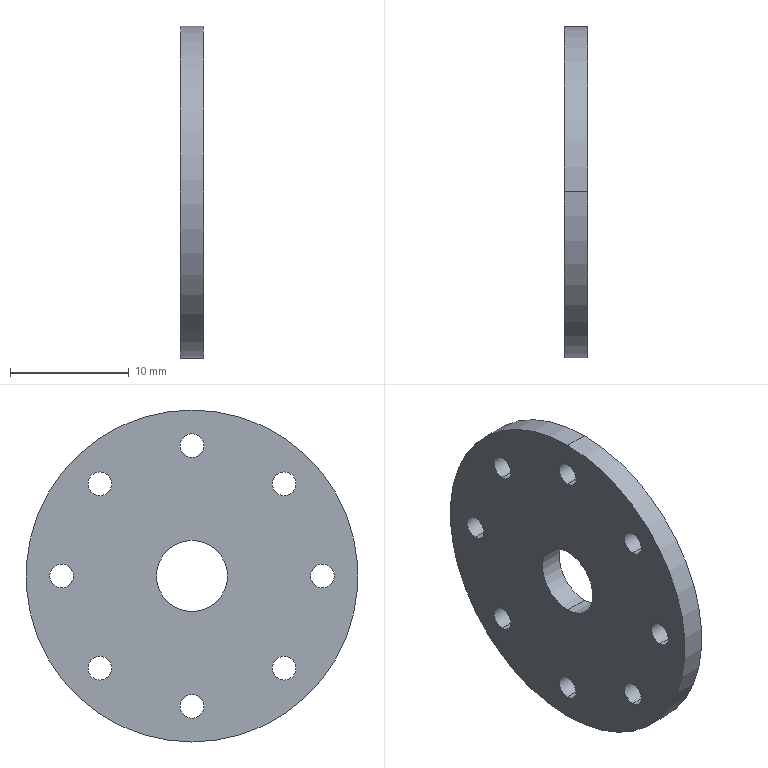Part | SolidWorks | features BaseBody 1 | 1 solid | 22 faces | box 2 x 28 x 28 mm | volume 1125 mm3 | cylinder 20 | plane 2 | commonest cylinder face diameters 2 x16 6 x2 28 x2
STEP:
#1=CARTESIAN_POINT('',(-2.,7.778,8.778));
#2=VERTEX_POINT('',#1);
#3=CARTESIAN_POINT('',(-2.,7.778,6.778));
#4=VERTEX_POINT('',#3);
#5=CARTESIAN_POINT('',(-2.,7.778,7.778));
#6=DIRECTION('',(1.,0.,0.));
#7=DIRECTION('',(0.,0.7071,-0.7071));
#8=AXIS2_PLACEMENT_3D('',#5,#6,#7);
#9=CIRCLE('',#8,1.);
#10=EDGE_CURVE('',#2,#4,#9,.T.);
#11=ORIENTED_EDGE('',*,*,#10,.F.);
#12=CARTESIAN_POINT('',(0.,7.778,8.778));
#13=VERTEX_POINT('',#12);
#14=CARTESIAN_POINT('',(-2.,7.778,8.778));
#15=DIRECTION('',(1.,0.,0.));
#16=VECTOR('',#15,1000.);
#17=LINE('',#14,#16);
#18=EDGE_CURVE('',#2,#13,#17,.T.);
#19=ORIENTED_EDGE('',*,*,#18,.T.);
#20=CARTESIAN_POINT('',(0.,7.778,6.778));
#21=VERTEX_POINT('',#20);
#22=CARTESIAN_POINT('',(0.,7.778,7.778));
#23=DIRECTION('',(1.,0.,0.));
#24=DIRECTION('',(0.,0.7071,-0.7071));
#25=AXIS2_PLACEMENT_3D('',#22,#23,#24);
#26=CIRCLE('',#25,1.);
#27=EDGE_CURVE('',#13,#21,#26,.T.);
#28=ORIENTED_EDGE('',*,*,#27,.T.);
#29=CARTESIAN_POINT('',(-2.,7.778,6.778));
#30=DIRECTION('',(1.,0.,0.));
#31=VECTOR('',#30,1000.);
#32=LINE('',#29,#31);
#33=EDGE_CURVE('',#4,#21,#32,.T.);
#34=ORIENTED_EDGE('',*,*,#33,.F.);
#35=EDGE_LOOP('',(#11,#19,#28,#34));
#36=FACE_OUTER_BOUND('',#35,.T.);
#37=CARTESIAN_POINT('',(-2.,7.778,7.778));
#38=DIRECTION('',(1.,0.,0.));
#39=DIRECTION('',(0.,0.,-1.));
#40=AXIS2_PLACEMENT_3D('',#37,#38,#39);
#41=CYLINDRICAL_SURFACE('',#40,1.);
#42=ADVANCED_FACE('',(#36),#41,.F.);
#43=CARTESIAN_POINT('',(-2.,0.,12.));
#44=VERTEX_POINT('',#43);
#45=CARTESIAN_POINT('',(-2.,0.,10.));
#46=VERTEX_POINT('',#45);
#47=CARTESIAN_POINT('',(-2.,0.,11.));
#48=DIRECTION('',(1.,0.,0.));
#49=DIRECTION('',(0.,1.,0.));
#50=AXIS2_PLACEMENT_3D('',#47,#48,#49);
#51=CIRCLE('',#50,1.);
#52=EDGE_CURVE('',#44,#46,#51,.T.);
#53=ORIENTED_EDGE('',*,*,#52,.F.);
#54=CARTESIAN_POINT('',(0.,0.,12.));
#55=VERTEX_POINT('',#54);
#56=CARTESIAN_POINT('',(-2.,0.,12.));
#57=DIRECTION('',(1.,0.,0.));
#58=VECTOR('',#57,1000.);
#59=LINE('',#56,#58);
#60=EDGE_CURVE('',#44,#55,#59,.T.);
#61=ORIENTED_EDGE('',*,*,#60,.T.);
#62=CARTESIAN_POINT('',(0.,0.,10.));
#63=VERTEX_POINT('',#62);
#64=CARTESIAN_POINT('',(0.,0.,11.));
#65=DIRECTION('',(1.,0.,0.));
#66=DIRECTION('',(0.,1.,0.));
#67=AXIS2_PLACEMENT_3D('',#64,#65,#66);
#68=CIRCLE('',#67,1.);
#69=EDGE_CURVE('',#55,#63,#68,.T.);
#70=ORIENTED_EDGE('',*,*,#69,.T.);
#71=CARTESIAN_POINT('',(-2.,0.,10.));
#72=DIRECTION('',(1.,0.,0.));
#73=VECTOR('',#72,1000.);
#74=LINE('',#71,#73);
#75=EDGE_CURVE('',#46,#63,#74,.T.);
#76=ORIENTED_EDGE('',*,*,#75,.F.);
#77=EDGE_LOOP('',(#53,#61,#70,#76));
#78=FACE_OUTER_BOUND('',#77,.T.);
#79=CARTESIAN_POINT('',(-2.,0.,11.));
#80=DIRECTION('',(1.,0.,0.));
#81=DIRECTION('',(0.,0.,-1.));
#82=AXIS2_PLACEMENT_3D('',#79,#80,#81);
#83=CYLINDRICAL_SURFACE('',#82,1.);
#84=ADVANCED_FACE('',(#78),#83,.F.);
#85=CARTESIAN_POINT('',(-2.,-7.778,8.778));
#86=VERTEX_POINT('',#85);
#87=CARTESIAN_POINT('',(-2.,-7.778,6.778));
#88=VERTEX_POINT('',#87);
#89=CARTESIAN_POINT('',(-2.,-7.778,7.778));
#90=DIRECTION('',(1.,0.,0.));
#91=DIRECTION('',(0.,0.7071,0.7071));
#92=AXIS2_PLACEMENT_3D('',#89,#90,#91);
#93=CIRCLE('',#92,1.);
#94=EDGE_CURVE('',#86,#88,#93,.T.);
#95=ORIENTED_EDGE('',*,*,#94,.F.);
#96=CARTESIAN_POINT('',(0.,-7.778,8.778));
#97=VERTEX_POINT('',#96);
#98=CARTESIAN_POINT('',(-2.,-7.778,8.778));
#99=DIRECTION('',(1.,0.,0.));
#100=VECTOR('',#99,1000.);
#101=LINE('',#98,#100);
#102=EDGE_CURVE('',#86,#97,#101,.T.);
#103=ORIENTED_EDGE('',*,*,#102,.T.);
#104=CARTESIAN_POINT('',(0.,-7.778,6.778));
#105=VERTEX_POINT('',#104);
#106=CARTESIAN_POINT('',(0.,-7.778,7.778));
#107=DIRECTION('',(1.,0.,0.));
#108=DIRECTION('',(0.,0.7071,0.7071));
#109=AXIS2_PLACEMENT_3D('',#106,#107,#108);
#110=CIRCLE('',#109,1.);
#111=EDGE_CURVE('',#97,#105,#110,.T.);
#112=ORIENTED_EDGE('',*,*,#111,.T.);
#113=CARTESIAN_POINT('',(-2.,-7.778,6.778));
#114=DIRECTION('',(1.,0.,0.));
#115=VECTOR('',#114,1000.);
#116=LINE('',#113,#115);
#117=EDGE_CURVE('',#88,#105,#116,.T.);
#118=ORIENTED_EDGE('',*,*,#117,.F.);
#119=EDGE_LOOP('',(#95,#103,#112,#118));
#120=FACE_OUTER_BOUND('',#119,.T.);
#121=CARTESIAN_POINT('',(-2.,-7.778,7.778));
#122=DIRECTION('',(1.,0.,0.));
#123=DIRECTION('',(0.,0.,-1.));
#124=AXIS2_PLACEMENT_3D('',#121,#122,#123);
#125=CYLINDRICAL_SURFACE('',#124,1.);
#126=ADVANCED_FACE('',(#120),#125,.F.);
#127=CARTESIAN_POINT('',(-2.,-11.,1.));
#128=VERTEX_POINT('',#127);
#129=CARTESIAN_POINT('',(-2.,-11.,-1.));
#130=VERTEX_POINT('',#129);
#131=CARTESIAN_POINT('',(-2.,-11.,0.));
#132=DIRECTION('',(1.,0.,0.));
#133=DIRECTION('',(0.,0.,1.));
#134=AXIS2_PLACEMENT_3D('',#131,#132,#133);
#135=CIRCLE('',#134,1.);
#136=EDGE_CURVE('',#128,#130,#135,.T.);
#137=ORIENTED_EDGE('',*,*,#136,.F.);
#138=CARTESIAN_POINT('',(0.,-11.,1.));
#139=VERTEX_POINT('',#138);
#140=CARTESIAN_POINT('',(-2.,-11.,1.));
#141=DIRECTION('',(1.,0.,0.));
#142=VECTOR('',#141,1000.);
#143=LINE('',#140,#142);
#144=EDGE_CURVE('',#128,#139,#143,.T.);
#145=ORIENTED_EDGE('',*,*,#144,.T.);
#146=CARTESIAN_POINT('',(0.,-11.,-1.));
#147=VERTEX_POINT('',#146);
#148=CARTESIAN_POINT('',(0.,-11.,0.));
#149=DIRECTION('',(1.,0.,0.));
#150=DIRECTION('',(0.,0.,1.));
#151=AXIS2_PLACEMENT_3D('',#148,#149,#150);
#152=CIRCLE('',#151,1.);
#153=EDGE_CURVE('',#139,#147,#152,.T.);
#154=ORIENTED_EDGE('',*,*,#153,.T.);
#155=CARTESIAN_POINT('',(-2.,-11.,-1.));
#156=DIRECTION('',(1.,0.,0.));
#157=VECTOR('',#156,1000.);
#158=LINE('',#155,#157);
#159=EDGE_CURVE('',#130,#147,#158,.T.);
#160=ORIENTED_EDGE('',*,*,#159,.F.);
#161=EDGE_LOOP('',(#137,#145,#154,#160));
#162=FACE_OUTER_BOUND('',#161,.T.);
#163=CARTESIAN_POINT('',(-2.,-11.,0.));
#164=DIRECTION('',(1.,0.,0.));
#165=DIRECTION('',(0.,0.,-1.));
#166=AXIS2_PLACEMENT_3D('',#163,#164,#165);
#167=CYLINDRICAL_SURFACE('',#166,1.);
#168=ADVANCED_FACE('',(#162),#167,.F.);
#169=CARTESIAN_POINT('',(-2.,-7.778,-6.778));
#170=VERTEX_POINT('',#169);
#171=CARTESIAN_POINT('',(-2.,-7.778,-8.778));
#172=VERTEX_POINT('',#171);
#173=CARTESIAN_POINT('',(-2.,-7.778,-7.778));
#174=DIRECTION('',(1.,0.,0.));
#175=DIRECTION('',(0.,-0.7071,0.7071));
#176=AXIS2_PLACEMENT_3D('',#173,#174,#175);
#177=CIRCLE('',#176,1.);
#178=EDGE_CURVE('',#170,#172,#177,.T.);
#179=ORIENTED_EDGE('',*,*,#178,.F.);
#180=CARTESIAN_POINT('',(0.,-7.778,-6.778));
#181=VERTEX_POINT('',#180);
#182=CARTESIAN_POINT('',(-2.,-7.778,-6.778));
#183=DIRECTION('',(1.,0.,0.));
#184=VECTOR('',#183,1000.);
#185=LINE('',#182,#184);
#186=EDGE_CURVE('',#170,#181,#185,.T.);
#187=ORIENTED_EDGE('',*,*,#186,.T.);
#188=CARTESIAN_POINT('',(0.,-7.778,-8.778));
#189=VERTEX_POINT('',#188);
#190=CARTESIAN_POINT('',(0.,-7.778,-7.778));
#191=DIRECTION('',(1.,0.,0.));
#192=DIRECTION('',(0.,-0.7071,0.7071));
#193=AXIS2_PLACEMENT_3D('',#190,#191,#192);
#194=CIRCLE('',#193,1.);
#195=EDGE_CURVE('',#181,#189,#194,.T.);
#196=ORIENTED_EDGE('',*,*,#195,.T.);
#197=CARTESIAN_POINT('',(-2.,-7.778,-8.778));
#198=DIRECTION('',(1.,0.,0.));
#199=VECTOR('',#198,1000.);
#200=LINE('',#197,#199);
#201=EDGE_CURVE('',#172,#189,#200,.T.);
#202=ORIENTED_EDGE('',*,*,#201,.F.);
#203=EDGE_LOOP('',(#179,#187,#196,#202));
#204=FACE_OUTER_BOUND('',#203,.T.);
#205=CARTESIAN_POINT('',(-2.,-7.778,-7.778));
#206=DIRECTION('',(1.,0.,0.));
#207=DIRECTION('',(0.,0.,-1.));
#208=AXIS2_PLACEMENT_3D('',#205,#206,#207);
#209=CYLINDRICAL_SURFACE('',#208,1.);
#210=ADVANCED_FACE('',(#204),#209,.F.);
#211=CARTESIAN_POINT('',(-2.,0.,-10.));
#212=VERTEX_POINT('',#211);
#213=CARTESIAN_POINT('',(-2.,0.,-12.));
#214=VERTEX_POINT('',#213);
#215=CARTESIAN_POINT('',(-2.,0.,-11.));
#216=DIRECTION('',(1.,0.,0.));
#217=DIRECTION('',(0.,-1.,0.));
#218=AXIS2_PLACEMENT_3D('',#215,#216,#217);
#219=CIRCLE('',#218,1.);
#220=EDGE_CURVE('',#212,#214,#219,.T.);
#221=ORIENTED_EDGE('',*,*,#220,.F.);
#222=CARTESIAN_POINT('',(0.,0.,-10.));
#223=VERTEX_POINT('',#222);
#224=CARTESIAN_POINT('',(-2.,0.,-10.));
#225=DIRECTION('',(1.,0.,0.));
#226=VECTOR('',#225,1000.);
#227=LINE('',#224,#226);
#228=EDGE_CURVE('',#212,#223,#227,.T.);
#229=ORIENTED_EDGE('',*,*,#228,.T.);
#230=CARTESIAN_POINT('',(0.,0.,-12.));
#231=VERTEX_POINT('',#230);
#232=CARTESIAN_POINT('',(0.,0.,-11.));
#233=DIRECTION('',(1.,0.,0.));
#234=DIRECTION('',(0.,-1.,0.));
#235=AXIS2_PLACEMENT_3D('',#232,#233,#234);
#236=CIRCLE('',#235,1.);
#237=EDGE_CURVE('',#223,#231,#236,.T.);
#238=ORIENTED_EDGE('',*,*,#237,.T.);
#239=CARTESIAN_POINT('',(-2.,0.,-12.));
#240=DIRECTION('',(1.,0.,0.));
#241=VECTOR('',#240,1000.);
#242=LINE('',#239,#241);
#243=EDGE_CURVE('',#214,#231,#242,.T.);
#244=ORIENTED_EDGE('',*,*,#243,.F.);
#245=EDGE_LOOP('',(#221,#229,#238,#244));
#246=FACE_OUTER_BOUND('',#245,.T.);
#247=CARTESIAN_POINT('',(-2.,0.,-11.));
#248=DIRECTION('',(1.,0.,0.));
#249=DIRECTION('',(0.,0.,-1.));
#250=AXIS2_PLACEMENT_3D('',#247,#248,#249);
#251=CYLINDRICAL_SURFACE('',#250,1.);
#252=ADVANCED_FACE('',(#246),#251,.F.);
#253=CARTESIAN_POINT('',(-2.,7.778,-6.778));
#254=VERTEX_POINT('',#253);
#255=CARTESIAN_POINT('',(-2.,7.778,-8.778));
#256=VERTEX_POINT('',#255);
#257=CARTESIAN_POINT('',(-2.,7.778,-7.778));
#258=DIRECTION('',(1.,0.,0.));
#259=DIRECTION('',(0.,-0.7071,-0.7071));
#260=AXIS2_PLACEMENT_3D('',#257,#258,#259);
#261=CIRCLE('',#260,1.);
#262=EDGE_CURVE('',#254,#256,#261,.T.);
#263=ORIENTED_EDGE('',*,*,#262,.F.);
#264=CARTESIAN_POINT('',(0.,7.778,-6.778));
#265=VERTEX_POINT('',#264);
#266=CARTESIAN_POINT('',(-2.,7.778,-6.778));
#267=DIRECTION('',(1.,0.,0.));
#268=VECTOR('',#267,1000.);
#269=LINE('',#266,#268);
#270=EDGE_CURVE('',#254,#265,#269,.T.);
#271=ORIENTED_EDGE('',*,*,#270,.T.);
#272=CARTESIAN_POINT('',(0.,7.778,-8.778));
#273=VERTEX_POINT('',#272);
#274=CARTESIAN_POINT('',(0.,7.778,-7.778));
#275=DIRECTION('',(1.,0.,0.));
#276=DIRECTION('',(0.,-0.7071,-0.7071));
#277=AXIS2_PLACEMENT_3D('',#274,#275,#276);
#278=CIRCLE('',#277,1.);
#279=EDGE_CURVE('',#265,#273,#278,.T.);
#280=ORIENTED_EDGE('',*,*,#279,.T.);
#281=CARTESIAN_POINT('',(-2.,7.778,-8.778));
#282=DIRECTION('',(1.,0.,0.));
#283=VECTOR('',#282,1000.);
#284=LINE('',#281,#283);
#285=EDGE_CURVE('',#256,#273,#284,.T.);
#286=ORIENTED_EDGE('',*,*,#285,.F.);
#287=EDGE_LOOP('',(#263,#271,#280,#286));
#288=FACE_OUTER_BOUND('',#287,.T.);
#289=CARTESIAN_POINT('',(-2.,7.778,-7.778));
#290=DIRECTION('',(1.,0.,0.));
#291=DIRECTION('',(0.,0.,-1.));
#292=AXIS2_PLACEMENT_3D('',#289,#290,#291);
#293=CYLINDRICAL_SURFACE('',#292,1.);
#294=ADVANCED_FACE('',(#288),#293,.F.);
#295=CARTESIAN_POINT('',(-2.,11.,1.));
#296=VERTEX_POINT('',#295);
#297=CARTESIAN_POINT('',(-2.,11.,-1.));
#298=VERTEX_POINT('',#297);
#299=CARTESIAN_POINT('',(-2.,11.,0.));
#300=DIRECTION('',(1.,0.,0.));
#301=DIRECTION('',(0.,0.,-1.));
#302=AXIS2_PLACEMENT_3D('',#299,#300,#301);
#303=CIRCLE('',#302,1.);
#304=EDGE_CURVE('',#296,#298,#303,.T.);
#305=ORIENTED_EDGE('',*,*,#304,.F.);
#306=CARTESIAN_POINT('',(0.,11.,1.));
#307=VERTEX_POINT('',#306);
#308=CARTESIAN_POINT('',(-2.,11.,1.));
#309=DIRECTION('',(1.,0.,0.));
#310=VECTOR('',#309,1000.);
#311=LINE('',#308,#310);
#312=EDGE_CURVE('',#296,#307,#311,.T.);
#313=ORIENTED_EDGE('',*,*,#312,.T.);
#314=CARTESIAN_POINT('',(0.,11.,-1.));
#315=VERTEX_POINT('',#314);
#316=CARTESIAN_POINT('',(0.,11.,0.));
#317=DIRECTION('',(1.,0.,0.));
#318=DIRECTION('',(0.,0.,-1.));
#319=AXIS2_PLACEMENT_3D('',#316,#317,#318);
#320=CIRCLE('',#319,1.);
#321=EDGE_CURVE('',#307,#315,#320,.T.);
#322=ORIENTED_EDGE('',*,*,#321,.T.);
#323=CARTESIAN_POINT('',(-2.,11.,-1.));
#324=DIRECTION('',(1.,0.,0.));
#325=VECTOR('',#324,1000.);
#326=LINE('',#323,#325);
#327=EDGE_CURVE('',#298,#315,#326,.T.);
#328=ORIENTED_EDGE('',*,*,#327,.F.);
#329=EDGE_LOOP('',(#305,#313,#322,#328));
#330=FACE_OUTER_BOUND('',#329,.T.);
#331=CARTESIAN_POINT('',(-2.,11.,0.));
#332=DIRECTION('',(1.,0.,0.));
#333=DIRECTION('',(0.,0.,-1.));
#334=AXIS2_PLACEMENT_3D('',#331,#332,#333);
#335=CYLINDRICAL_SURFACE('',#334,1.);
#336=ADVANCED_FACE('',(#330),#335,.F.);
#337=CARTESIAN_POINT('',(0.,0.,-3.));
#338=VERTEX_POINT('',#337);
#339=CARTESIAN_POINT('',(0.,0.,3.));
#340=VERTEX_POINT('',#339);
#341=CARTESIAN_POINT('',(0.,0.,0.));
#342=DIRECTION('',(-1.,0.,0.));
#343=DIRECTION('',(0.,0.,1.));
#344=AXIS2_PLACEMENT_3D('',#341,#342,#343);
#345=CIRCLE('',#344,3.);
#346=EDGE_CURVE('',#338,#340,#345,.T.);
#347=ORIENTED_EDGE('',*,*,#346,.F.);
#348=CARTESIAN_POINT('',(-2.,0.,-3.));
#349=VERTEX_POINT('',#348);
#350=CARTESIAN_POINT('',(0.,0.,-3.));
#351=DIRECTION('',(-1.,0.,0.));
#352=VECTOR('',#351,1000.);
#353=LINE('',#350,#352);
#354=EDGE_CURVE('',#338,#349,#353,.T.);
#355=ORIENTED_EDGE('',*,*,#354,.T.);
#356=CARTESIAN_POINT('',(-2.,0.,3.));
#357=VERTEX_POINT('',#356);
#358=CARTESIAN_POINT('',(-2.,0.,0.));
#359=DIRECTION('',(-1.,0.,0.));
#360=DIRECTION('',(0.,0.,1.));
#361=AXIS2_PLACEMENT_3D('',#358,#359,#360);
#362=CIRCLE('',#361,3.);
#363=EDGE_CURVE('',#349,#357,#362,.T.);
#364=ORIENTED_EDGE('',*,*,#363,.T.);
#365=CARTESIAN_POINT('',(0.,0.,3.));
#366=DIRECTION('',(-1.,0.,0.));
#367=VECTOR('',#366,1000.);
#368=LINE('',#365,#367);
#369=EDGE_CURVE('',#340,#357,#368,.T.);
#370=ORIENTED_EDGE('',*,*,#369,.F.);
#371=EDGE_LOOP('',(#347,#355,#364,#370));
#372=FACE_OUTER_BOUND('',#371,.T.);
#373=CARTESIAN_POINT('',(0.,0.,0.));
#374=DIRECTION('',(-1.,0.,0.));
#375=DIRECTION('',(0.,0.,1.));
#376=AXIS2_PLACEMENT_3D('',#373,#374,#375);
#377=CYLINDRICAL_SURFACE('',#376,3.);
#378=ADVANCED_FACE('',(#372),#377,.F.);
#379=CARTESIAN_POINT('',(0.,0.,14.));
#380=VERTEX_POINT('',#379);
#381=CARTESIAN_POINT('',(0.,0.,-14.));
#382=VERTEX_POINT('',#381);
#383=CARTESIAN_POINT('',(0.,0.,0.));
#384=DIRECTION('',(-1.,0.,0.));
#385=DIRECTION('',(0.,0.,1.));
#386=AXIS2_PLACEMENT_3D('',#383,#384,#385);
#387=CIRCLE('',#386,14.);
#388=EDGE_CURVE('',#380,#382,#387,.T.);
#389=ORIENTED_EDGE('',*,*,#388,.T.);
#390=CARTESIAN_POINT('',(-2.,0.,-14.));
#391=VERTEX_POINT('',#390);
#392=CARTESIAN_POINT('',(0.,0.,-14.));
#393=DIRECTION('',(-1.,0.,0.));
#394=VECTOR('',#393,1000.);
#395=LINE('',#392,#394);
#396=EDGE_CURVE('',#382,#391,#395,.T.);
#397=ORIENTED_EDGE('',*,*,#396,.T.);
#398=CARTESIAN_POINT('',(-2.,0.,14.));
#399=VERTEX_POINT('',#398);
#400=CARTESIAN_POINT('',(-2.,0.,0.));
#401=DIRECTION('',(-1.,0.,0.));
#402=DIRECTION('',(0.,0.,1.));
#403=AXIS2_PLACEMENT_3D('',#400,#401,#402);
#404=CIRCLE('',#403,14.);
#405=EDGE_CURVE('',#399,#391,#404,.T.);
#406=ORIENTED_EDGE('',*,*,#405,.F.);
#407=CARTESIAN_POINT('',(0.,0.,14.));
#408=DIRECTION('',(-1.,0.,0.));
#409=VECTOR('',#408,1000.);
#410=LINE('',#407,#409);
#411=EDGE_CURVE('',#380,#399,#410,.T.);
#412=ORIENTED_EDGE('',*,*,#411,.F.);
#413=EDGE_LOOP('',(#389,#397,#406,#412));
#414=FACE_OUTER_BOUND('',#413,.T.);
#415=CARTESIAN_POINT('',(0.,0.,0.));
#416=DIRECTION('',(-1.,0.,0.));
#417=DIRECTION('',(0.,0.,1.));
#418=AXIS2_PLACEMENT_3D('',#415,#416,#417);
#419=CYLINDRICAL_SURFACE('',#418,14.);
#420=ADVANCED_FACE('',(#414),#419,.T.);
#421=CARTESIAN_POINT('',(-2.,7.778,7.778));
#422=DIRECTION('',(1.,0.,0.));
#423=DIRECTION('',(0.,0.7071,-0.7071));
#424=AXIS2_PLACEMENT_3D('',#421,#422,#423);
#425=CIRCLE('',#424,1.);
#426=EDGE_CURVE('',#4,#2,#425,.T.);
#427=ORIENTED_EDGE('',*,*,#426,.T.);
#428=ORIENTED_EDGE('',*,*,#10,.T.);
#429=EDGE_LOOP('',(#427,#428));
#430=FACE_BOUND('',#429,.T.);
#431=CARTESIAN_POINT('',(-2.,0.,11.));
#432=DIRECTION('',(1.,0.,0.));
#433=DIRECTION('',(0.,1.,0.));
#434=AXIS2_PLACEMENT_3D('',#431,#432,#433);
#435=CIRCLE('',#434,1.);
#436=EDGE_CURVE('',#46,#44,#435,.T.);
#437=ORIENTED_EDGE('',*,*,#436,.T.);
#438=ORIENTED_EDGE('',*,*,#52,.T.);
#439=EDGE_LOOP('',(#437,#438));
#440=FACE_BOUND('',#439,.T.);
#441=CARTESIAN_POINT('',(-2.,-7.778,7.778));
#442=DIRECTION('',(1.,0.,0.));
#443=DIRECTION('',(0.,0.7071,0.7071));
#444=AXIS2_PLACEMENT_3D('',#441,#442,#443);
#445=CIRCLE('',#444,1.);
#446=EDGE_CURVE('',#88,#86,#445,.T.);
#447=ORIENTED_EDGE('',*,*,#446,.T.);
#448=ORIENTED_EDGE('',*,*,#94,.T.);
#449=EDGE_LOOP('',(#447,#448));
#450=FACE_BOUND('',#449,.T.);
#451=CARTESIAN_POINT('',(-2.,-11.,0.));
#452=DIRECTION('',(1.,0.,0.));
#453=DIRECTION('',(0.,0.,1.));
#454=AXIS2_PLACEMENT_3D('',#451,#452,#453);
#455=CIRCLE('',#454,1.);
#456=EDGE_CURVE('',#130,#128,#455,.T.);
#457=ORIENTED_EDGE('',*,*,#456,.T.);
#458=ORIENTED_EDGE('',*,*,#136,.T.);
#459=EDGE_LOOP('',(#457,#458));
#460=FACE_BOUND('',#459,.T.);
#461=CARTESIAN_POINT('',(-2.,-7.778,-7.778));
#462=DIRECTION('',(1.,0.,0.));
#463=DIRECTION('',(0.,-0.7071,0.7071));
#464=AXIS2_PLACEMENT_3D('',#461,#462,#463);
#465=CIRCLE('',#464,1.);
#466=EDGE_CURVE('',#172,#170,#465,.T.);
#467=ORIENTED_EDGE('',*,*,#466,.T.);
#468=ORIENTED_EDGE('',*,*,#178,.T.);
#469=EDGE_LOOP('',(#467,#468));
#470=FACE_BOUND('',#469,.T.);
#471=CARTESIAN_POINT('',(-2.,0.,-11.));
#472=DIRECTION('',(1.,0.,0.));
#473=DIRECTION('',(0.,-1.,0.));
#474=AXIS2_PLACEMENT_3D('',#471,#472,#473);
#475=CIRCLE('',#474,1.);
#476=EDGE_CURVE('',#214,#212,#475,.T.);
#477=ORIENTED_EDGE('',*,*,#476,.T.);
#478=ORIENTED_EDGE('',*,*,#220,.T.);
#479=EDGE_LOOP('',(#477,#478));
#480=FACE_BOUND('',#479,.T.);
#481=CARTESIAN_POINT('',(-2.,7.778,-7.778));
#482=DIRECTION('',(1.,0.,0.));
#483=DIRECTION('',(0.,-0.7071,-0.7071));
#484=AXIS2_PLACEMENT_3D('',#481,#482,#483);
#485=CIRCLE('',#484,1.);
#486=EDGE_CURVE('',#256,#254,#485,.T.);
#487=ORIENTED_EDGE('',*,*,#486,.T.);
#488=ORIENTED_EDGE('',*,*,#262,.T.);
#489=EDGE_LOOP('',(#487,#488));
#490=FACE_BOUND('',#489,.T.);
#491=CARTESIAN_POINT('',(-2.,11.,0.));
#492=DIRECTION('',(1.,0.,0.));
#493=DIRECTION('',(0.,0.,-1.));
#494=AXIS2_PLACEMENT_3D('',#491,#492,#493);
#495=CIRCLE('',#494,1.);
#496=EDGE_CURVE('',#298,#296,#495,.T.);
#497=ORIENTED_EDGE('',*,*,#496,.T.);
#498=ORIENTED_EDGE('',*,*,#304,.T.);
#499=EDGE_LOOP('',(#497,#498));
#500=FACE_BOUND('',#499,.T.);
#501=CARTESIAN_POINT('',(-2.,0.,0.));
#502=DIRECTION('',(-1.,0.,0.));
#503=DIRECTION('',(0.,0.,1.));
#504=AXIS2_PLACEMENT_3D('',#501,#502,#503);
#505=CIRCLE('',#504,3.);
#506=EDGE_CURVE('',#357,#349,#505,.T.);
#507=ORIENTED_EDGE('',*,*,#506,.F.);
#508=ORIENTED_EDGE('',*,*,#363,.F.);
#509=EDGE_LOOP('',(#507,#508));
#510=FACE_BOUND('',#509,.T.);
#511=ORIENTED_EDGE('',*,*,#405,.T.);
#512=CARTESIAN_POINT('',(-2.,0.,0.));
#513=DIRECTION('',(-1.,0.,0.));
#514=DIRECTION('',(0.,0.,1.));
#515=AXIS2_PLACEMENT_3D('',#512,#513,#514);
#516=CIRCLE('',#515,14.);
#517=EDGE_CURVE('',#391,#399,#516,.T.);
#518=ORIENTED_EDGE('',*,*,#517,.T.);
#519=EDGE_LOOP('',(#511,#518));
#520=FACE_OUTER_BOUND('',#519,.T.);
#521=CARTESIAN_POINT('',(-2.,3.,0.));
#522=DIRECTION('',(1.,0.,0.));
#523=DIRECTION('',(0.,0.,-1.));
#524=AXIS2_PLACEMENT_3D('',#521,#522,#523);
#525=PLANE('',#524);
#526=ADVANCED_FACE('',(#430,#440,#450,#460,#470,#480,#490,#500,#510,#520),#525,.F.);
#527=ORIENTED_EDGE('',*,*,#396,.F.);
#528=CARTESIAN_POINT('',(0.,0.,0.));
#529=DIRECTION('',(-1.,0.,0.));
#530=DIRECTION('',(0.,0.,1.));
#531=AXIS2_PLACEMENT_3D('',#528,#529,#530);
#532=CIRCLE('',#531,14.);
#533=EDGE_CURVE('',#382,#380,#532,.T.);
#534=ORIENTED_EDGE('',*,*,#533,.T.);
#535=ORIENTED_EDGE('',*,*,#411,.T.);
#536=ORIENTED_EDGE('',*,*,#517,.F.);
#537=EDGE_LOOP('',(#527,#534,#535,#536));
#538=FACE_OUTER_BOUND('',#537,.T.);
#539=CARTESIAN_POINT('',(0.,0.,0.));
#540=DIRECTION('',(-1.,0.,0.));
#541=DIRECTION('',(0.,0.,1.));
#542=AXIS2_PLACEMENT_3D('',#539,#540,#541);
#543=CYLINDRICAL_SURFACE('',#542,14.);
#544=ADVANCED_FACE('',(#538),#543,.T.);
#545=CARTESIAN_POINT('',(0.,7.778,7.778));
#546=DIRECTION('',(1.,0.,0.));
#547=DIRECTION('',(0.,0.7071,-0.7071));
#548=AXIS2_PLACEMENT_3D('',#545,#546,#547);
#549=CIRCLE('',#548,1.);
#550=EDGE_CURVE('',#21,#13,#549,.T.);
#551=ORIENTED_EDGE('',*,*,#550,.F.);
#552=ORIENTED_EDGE('',*,*,#27,.F.);
#553=EDGE_LOOP('',(#551,#552));
#554=FACE_BOUND('',#553,.T.);
#555=CARTESIAN_POINT('',(0.,0.,11.));
#556=DIRECTION('',(1.,0.,0.));
#557=DIRECTION('',(0.,1.,0.));
#558=AXIS2_PLACEMENT_3D('',#555,#556,#557);
#559=CIRCLE('',#558,1.);
#560=EDGE_CURVE('',#63,#55,#559,.T.);
#561=ORIENTED_EDGE('',*,*,#560,.F.);
#562=ORIENTED_EDGE('',*,*,#69,.F.);
#563=EDGE_LOOP('',(#561,#562));
#564=FACE_BOUND('',#563,.T.);
#565=CARTESIAN_POINT('',(0.,-7.778,7.778));
#566=DIRECTION('',(1.,0.,0.));
#567=DIRECTION('',(0.,0.7071,0.7071));
#568=AXIS2_PLACEMENT_3D('',#565,#566,#567);
#569=CIRCLE('',#568,1.);
#570=EDGE_CURVE('',#105,#97,#569,.T.);
#571=ORIENTED_EDGE('',*,*,#570,.F.);
#572=ORIENTED_EDGE('',*,*,#111,.F.);
#573=EDGE_LOOP('',(#571,#572));
#574=FACE_BOUND('',#573,.T.);
#575=CARTESIAN_POINT('',(0.,-11.,0.));
#576=DIRECTION('',(1.,0.,0.));
#577=DIRECTION('',(0.,0.,1.));
#578=AXIS2_PLACEMENT_3D('',#575,#576,#577);
#579=CIRCLE('',#578,1.);
#580=EDGE_CURVE('',#147,#139,#579,.T.);
#581=ORIENTED_EDGE('',*,*,#580,.F.);
#582=ORIENTED_EDGE('',*,*,#153,.F.);
#583=EDGE_LOOP('',(#581,#582));
#584=FACE_BOUND('',#583,.T.);
#585=CARTESIAN_POINT('',(0.,-7.778,-7.778));
#586=DIRECTION('',(1.,0.,0.));
#587=DIRECTION('',(0.,-0.7071,0.7071));
#588=AXIS2_PLACEMENT_3D('',#585,#586,#587);
#589=CIRCLE('',#588,1.);
#590=EDGE_CURVE('',#189,#181,#589,.T.);
#591=ORIENTED_EDGE('',*,*,#590,.F.);
#592=ORIENTED_EDGE('',*,*,#195,.F.);
#593=EDGE_LOOP('',(#591,#592));
#594=FACE_BOUND('',#593,.T.);
#595=CARTESIAN_POINT('',(0.,0.,-11.));
#596=DIRECTION('',(1.,0.,0.));
#597=DIRECTION('',(0.,-1.,0.));
#598=AXIS2_PLACEMENT_3D('',#595,#596,#597);
#599=CIRCLE('',#598,1.);
#600=EDGE_CURVE('',#231,#223,#599,.T.);
#601=ORIENTED_EDGE('',*,*,#600,.F.);
#602=ORIENTED_EDGE('',*,*,#237,.F.);
#603=EDGE_LOOP('',(#601,#602));
#604=FACE_BOUND('',#603,.T.);
#605=CARTESIAN_POINT('',(0.,7.778,-7.778));
#606=DIRECTION('',(1.,0.,0.));
#607=DIRECTION('',(0.,-0.7071,-0.7071));
#608=AXIS2_PLACEMENT_3D('',#605,#606,#607);
#609=CIRCLE('',#608,1.);
#610=EDGE_CURVE('',#273,#265,#609,.T.);
#611=ORIENTED_EDGE('',*,*,#610,.F.);
#612=ORIENTED_EDGE('',*,*,#279,.F.);
#613=EDGE_LOOP('',(#611,#612));
#614=FACE_BOUND('',#613,.T.);
#615=CARTESIAN_POINT('',(0.,11.,0.));
#616=DIRECTION('',(1.,0.,0.));
#617=DIRECTION('',(0.,0.,-1.));
#618=AXIS2_PLACEMENT_3D('',#615,#616,#617);
#619=CIRCLE('',#618,1.);
#620=EDGE_CURVE('',#315,#307,#619,.T.);
#621=ORIENTED_EDGE('',*,*,#620,.F.);
#622=ORIENTED_EDGE('',*,*,#321,.F.);
#623=EDGE_LOOP('',(#621,#622));
#624=FACE_BOUND('',#623,.T.);
#625=ORIENTED_EDGE('',*,*,#388,.F.);
#626=ORIENTED_EDGE('',*,*,#533,.F.);
#627=EDGE_LOOP('',(#625,#626));
#628=FACE_OUTER_BOUND('',#627,.T.);
#629=CARTESIAN_POINT('',(0.,0.,0.));
#630=DIRECTION('',(-1.,0.,0.));
#631=DIRECTION('',(0.,0.,1.));
#632=AXIS2_PLACEMENT_3D('',#629,#630,#631);
#633=CIRCLE('',#632,3.);
#634=EDGE_CURVE('',#340,#338,#633,.T.);
#635=ORIENTED_EDGE('',*,*,#634,.T.);
#636=ORIENTED_EDGE('',*,*,#346,.T.);
#637=EDGE_LOOP('',(#635,#636));
#638=FACE_BOUND('',#637,.T.);
#639=CARTESIAN_POINT('',(0.,14.,0.));
#640=DIRECTION('',(-1.,0.,0.));
#641=DIRECTION('',(0.,0.,1.));
#642=AXIS2_PLACEMENT_3D('',#639,#640,#641);
#643=PLANE('',#642);
#644=ADVANCED_FACE('',(#554,#564,#574,#584,#594,#604,#614,#624,#628,#638),#643,.F.);
#645=ORIENTED_EDGE('',*,*,#354,.F.);
#646=ORIENTED_EDGE('',*,*,#634,.F.);
#647=ORIENTED_EDGE('',*,*,#369,.T.);
#648=ORIENTED_EDGE('',*,*,#506,.T.);
#649=EDGE_LOOP('',(#645,#646,#647,#648));
#650=FACE_OUTER_BOUND('',#649,.T.);
#651=CARTESIAN_POINT('',(0.,0.,0.));
#652=DIRECTION('',(-1.,0.,0.));
#653=DIRECTION('',(0.,0.,1.));
#654=AXIS2_PLACEMENT_3D('',#651,#652,#653);
#655=CYLINDRICAL_SURFACE('',#654,3.);
#656=ADVANCED_FACE('',(#650),#655,.F.);
#657=ORIENTED_EDGE('',*,*,#312,.F.);
#658=ORIENTED_EDGE('',*,*,#496,.F.);
#659=ORIENTED_EDGE('',*,*,#327,.T.);
#660=ORIENTED_EDGE('',*,*,#620,.T.);
#661=EDGE_LOOP('',(#657,#658,#659,#660));
#662=FACE_OUTER_BOUND('',#661,.T.);
#663=CARTESIAN_POINT('',(-2.,11.,0.));
#664=DIRECTION('',(1.,0.,0.));
#665=DIRECTION('',(0.,0.,-1.));
#666=AXIS2_PLACEMENT_3D('',#663,#664,#665);
#667=CYLINDRICAL_SURFACE('',#666,1.);
#668=ADVANCED_FACE('',(#662),#667,.F.);
#669=ORIENTED_EDGE('',*,*,#270,.F.);
#670=ORIENTED_EDGE('',*,*,#486,.F.);
#671=ORIENTED_EDGE('',*,*,#285,.T.);
#672=ORIENTED_EDGE('',*,*,#610,.T.);
#673=EDGE_LOOP('',(#669,#670,#671,#672));
#674=FACE_OUTER_BOUND('',#673,.T.);
#675=CARTESIAN_POINT('',(-2.,7.778,-7.778));
#676=DIRECTION('',(1.,0.,0.));
#677=DIRECTION('',(0.,0.,-1.));
#678=AXIS2_PLACEMENT_3D('',#675,#676,#677);
#679=CYLINDRICAL_SURFACE('',#678,1.);
#680=ADVANCED_FACE('',(#674),#679,.F.);
#681=ORIENTED_EDGE('',*,*,#228,.F.);
#682=ORIENTED_EDGE('',*,*,#476,.F.);
#683=ORIENTED_EDGE('',*,*,#243,.T.);
#684=ORIENTED_EDGE('',*,*,#600,.T.);
#685=EDGE_LOOP('',(#681,#682,#683,#684));
#686=FACE_OUTER_BOUND('',#685,.T.);
#687=CARTESIAN_POINT('',(-2.,0.,-11.));
#688=DIRECTION('',(1.,0.,0.));
#689=DIRECTION('',(0.,0.,-1.));
#690=AXIS2_PLACEMENT_3D('',#687,#688,#689);
#691=CYLINDRICAL_SURFACE('',#690,1.);
#692=ADVANCED_FACE('',(#686),#691,.F.);
#693=ORIENTED_EDGE('',*,*,#186,.F.);
#694=ORIENTED_EDGE('',*,*,#466,.F.);
#695=ORIENTED_EDGE('',*,*,#201,.T.);
#696=ORIENTED_EDGE('',*,*,#590,.T.);
#697=EDGE_LOOP('',(#693,#694,#695,#696));
#698=FACE_OUTER_BOUND('',#697,.T.);
#699=CARTESIAN_POINT('',(-2.,-7.778,-7.778));
#700=DIRECTION('',(1.,0.,0.));
#701=DIRECTION('',(0.,0.,-1.));
#702=AXIS2_PLACEMENT_3D('',#699,#700,#701);
#703=CYLINDRICAL_SURFACE('',#702,1.);
#704=ADVANCED_FACE('',(#698),#703,.F.);
#705=ORIENTED_EDGE('',*,*,#144,.F.);
#706=ORIENTED_EDGE('',*,*,#456,.F.);
#707=ORIENTED_EDGE('',*,*,#159,.T.);
#708=ORIENTED_EDGE('',*,*,#580,.T.);
#709=EDGE_LOOP('',(#705,#706,#707,#708));
#710=FACE_OUTER_BOUND('',#709,.T.);
#711=CARTESIAN_POINT('',(-2.,-11.,0.));
#712=DIRECTION('',(1.,0.,0.));
#713=DIRECTION('',(0.,0.,-1.));
#714=AXIS2_PLACEMENT_3D('',#711,#712,#713);
#715=CYLINDRICAL_SURFACE('',#714,1.);
#716=ADVANCED_FACE('',(#710),#715,.F.);
#717=ORIENTED_EDGE('',*,*,#102,.F.);
#718=ORIENTED_EDGE('',*,*,#446,.F.);
#719=ORIENTED_EDGE('',*,*,#117,.T.);
#720=ORIENTED_EDGE('',*,*,#570,.T.);
#721=EDGE_LOOP('',(#717,#718,#719,#720));
#722=FACE_OUTER_BOUND('',#721,.T.);
#723=CARTESIAN_POINT('',(-2.,-7.778,7.778));
#724=DIRECTION('',(1.,0.,0.));
#725=DIRECTION('',(0.,0.,-1.));
#726=AXIS2_PLACEMENT_3D('',#723,#724,#725);
#727=CYLINDRICAL_SURFACE('',#726,1.);
#728=ADVANCED_FACE('',(#722),#727,.F.);
#729=ORIENTED_EDGE('',*,*,#60,.F.);
#730=ORIENTED_EDGE('',*,*,#436,.F.);
#731=ORIENTED_EDGE('',*,*,#75,.T.);
#732=ORIENTED_EDGE('',*,*,#560,.T.);
#733=EDGE_LOOP('',(#729,#730,#731,#732));
#734=FACE_OUTER_BOUND('',#733,.T.);
#735=CARTESIAN_POINT('',(-2.,0.,11.));
#736=DIRECTION('',(1.,0.,0.));
#737=DIRECTION('',(0.,0.,-1.));
#738=AXIS2_PLACEMENT_3D('',#735,#736,#737);
#739=CYLINDRICAL_SURFACE('',#738,1.);
#740=ADVANCED_FACE('',(#734),#739,.F.);
#741=ORIENTED_EDGE('',*,*,#18,.F.);
#742=ORIENTED_EDGE('',*,*,#426,.F.);
#743=ORIENTED_EDGE('',*,*,#33,.T.);
#744=ORIENTED_EDGE('',*,*,#550,.T.);
#745=EDGE_LOOP('',(#741,#742,#743,#744));
#746=FACE_OUTER_BOUND('',#745,.T.);
#747=CARTESIAN_POINT('',(-2.,7.778,7.778));
#748=DIRECTION('',(1.,0.,0.));
#749=DIRECTION('',(0.,0.,-1.));
#750=AXIS2_PLACEMENT_3D('',#747,#748,#749);
#751=CYLINDRICAL_SURFACE('',#750,1.);
#752=ADVANCED_FACE('',(#746),#751,.F.);
#753=CLOSED_SHELL('',(#42,#84,#126,#168,#210,#252,#294,#336,#378,#420,#526,#544,#644,#656,#668,#680,#692,#704,#716,#728,#740,#752));
#754=MANIFOLD_SOLID_BREP('',#753);
#755=CARTESIAN_POINT('',(0.,0.,0.));
#756=DIRECTION('',(0.,0.,1.));
#757=DIRECTION('',(1.,0.,0.));
#758=AXIS2_PLACEMENT_3D('',#755,#756,#757);
#759=(LENGTH_UNIT()NAMED_UNIT(*)SI_UNIT(.MILLI.,.METRE.));
#760=UNCERTAINTY_MEASURE_WITH_UNIT(LENGTH_MEASURE(0.00001),#759,'','');
#761=(NAMED_UNIT(*)PLANE_ANGLE_UNIT()SI_UNIT($,.RADIAN.));
#762=(NAMED_UNIT(*)SI_UNIT($,.STERADIAN.)SOLID_ANGLE_UNIT());
#763=(GEOMETRIC_REPRESENTATION_CONTEXT(3)GLOBAL_UNCERTAINTY_ASSIGNED_CONTEXT((#760))GLOBAL_UNIT_ASSIGNED_CONTEXT((#759,#761,#762))REPRESENTATION_CONTEXT('',''));
#764=ADVANCED_BREP_SHAPE_REPRESENTATION('',(#754,#758),#763);